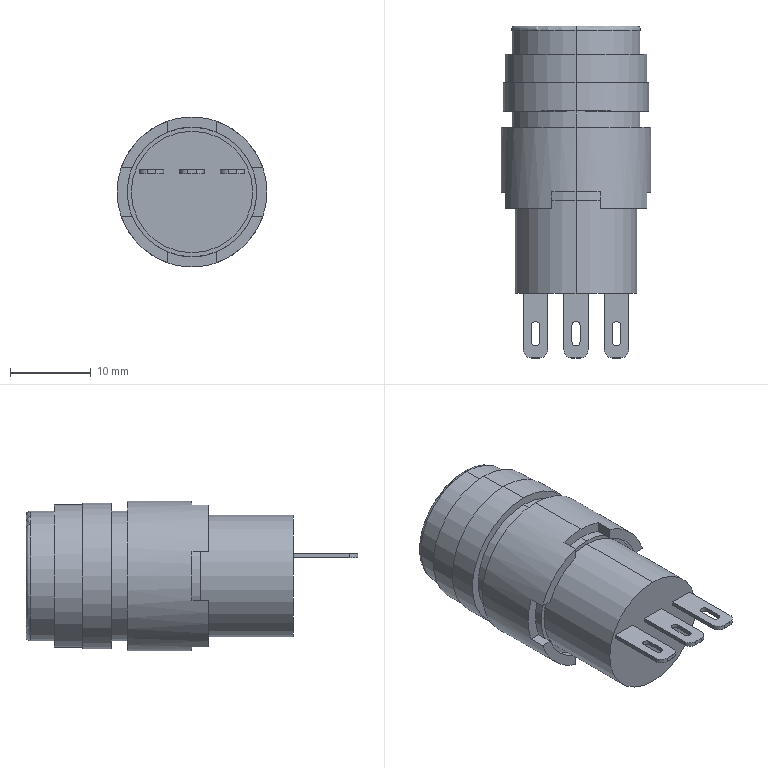Part | SolidWorks | features ICE 7, Fillet 2, CirPattern 1, Extrusion 1, RevCutThin 1 | 2 solids | 72 faces | box 18.5 x 41 x 18.5 mm | volume 7334 mm3 | plane 44 | cylinder 26 | torus 2 | commonest cylinder face diameters 1 x6 2 x6 16 x6 15 x2 17.6 x2 18 x2